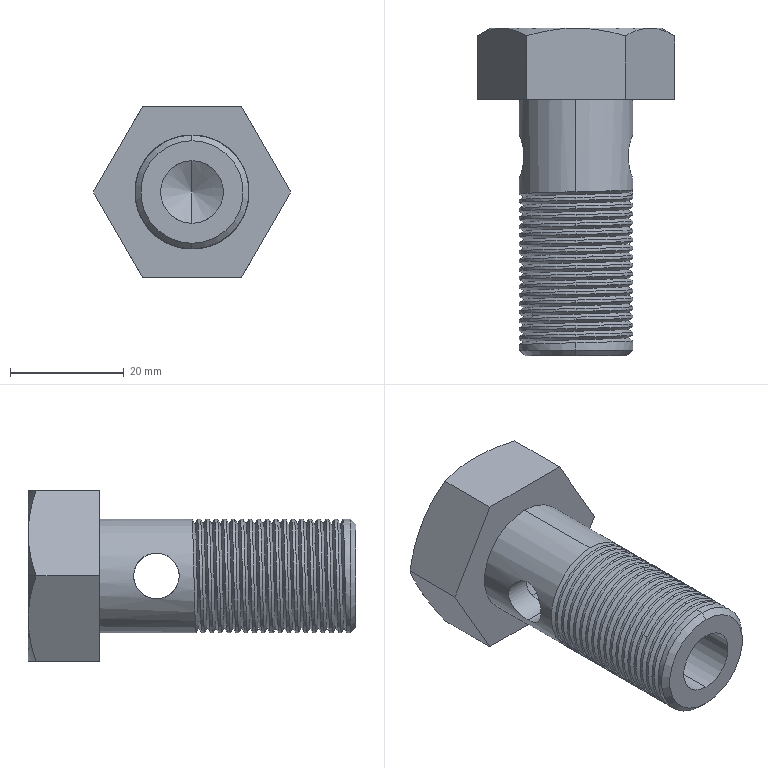Part | SolidWorks | features BaseBody 1 | 1 solid | 71 faces | box 34.64 x 57.5 x 29.999 mm | volume 18874 mm3 | cylinder 43 | plane 11 | spline 10 | cone 7 | commonest cylinder face diameters 20 x37 8 x4 11 x2